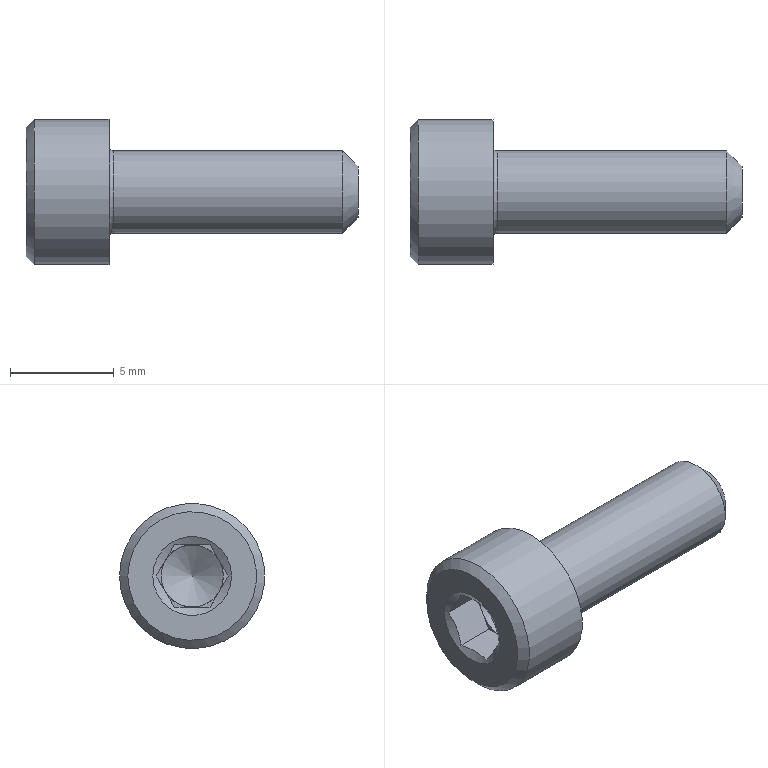Part | STEP file | Винт М4-6gx12 ГОСТ 11738-84 | 1 solid | 23 faces | box 16 x 7 x 7 mm | volume 277.854 mm3 | plane 15 | cone 4 | cylinder 3 | torus 1 | commonest cylinder face diameters 3 x1 4 x1 7 x1
STEP:
#1=CARTESIAN_POINT('',(-4.,3.1,0.));
#2=VERTEX_POINT('',#1);
#3=CARTESIAN_POINT('',(-4.,0.,0.));
#4=DIRECTION('',(1.,0.,0.));
#5=DIRECTION('',(0.,1.,0.));
#6=AXIS2_PLACEMENT_3D('',#3,#4,#5);
#7=CIRCLE('',#6,3.1);
#8=EDGE_CURVE('',#2,#2,#7,.T.);
#9=ORIENTED_EDGE('',*,*,#8,.F.);
#10=EDGE_LOOP('',(#9));
#11=FACE_BOUND('',#10,.T.);
#12=CARTESIAN_POINT('',(-4.,1.9,0.));
#13=VERTEX_POINT('',#12);
#14=CARTESIAN_POINT('',(-4.,0.,0.));
#15=DIRECTION('',(1.,0.,0.));
#16=DIRECTION('',(0.,1.,0.));
#17=AXIS2_PLACEMENT_3D('',#14,#15,#16);
#18=CIRCLE('',#17,1.9);
#19=EDGE_CURVE('',#13,#13,#18,.T.);
#20=ORIENTED_EDGE('',*,*,#19,.T.);
#21=EDGE_LOOP('',(#20));
#22=FACE_BOUND('',#21,.T.);
#23=CARTESIAN_POINT('',(-4.,0.,0.));
#24=DIRECTION('',(-1.,0.,0.));
#25=DIRECTION('',(0.,1.,0.));
#26=AXIS2_PLACEMENT_3D('',#23,#24,#25);
#27=PLANE('',#26);
#28=ADVANCED_FACE('',(#11,#22),#27,.T.);
#29=CARTESIAN_POINT('',(-3.903,0.866,-1.5));
#30=VERTEX_POINT('',#29);
#31=CARTESIAN_POINT('',(-3.903,-0.866,-1.5));
#32=VERTEX_POINT('',#31);
#33=CARTESIAN_POINT('',(-3.903,0.866,-1.5));
#34=CARTESIAN_POINT('',(-3.9,0.8561,-1.5));
#35=CARTESIAN_POINT('',(-3.89,0.8205,-1.5));
#36=CARTESIAN_POINT('',(-3.88,0.7841,-1.5));
#37=CARTESIAN_POINT('',(-3.862,0.7149,-1.5));
#38=CARTESIAN_POINT('',(-3.851,0.6675,-1.5));
#39=CARTESIAN_POINT('',(-3.83,0.5736,-1.5));
#40=CARTESIAN_POINT('',(-3.816,0.5059,-1.5));
#41=CARTESIAN_POINT('',(-3.8,0.4061,-1.5));
#42=CARTESIAN_POINT('',(-3.789,0.3305,-1.5));
#43=CARTESIAN_POINT('',(-3.781,0.2553,-1.5));
#44=CARTESIAN_POINT('',(-3.776,0.1888,-1.5));
#45=CARTESIAN_POINT('',(-3.773,0.1381,-1.5));
#46=CARTESIAN_POINT('',(-3.771,0.09396,-1.5));
#47=CARTESIAN_POINT('',(-3.77,0.0601,-1.5));
#48=CARTESIAN_POINT('',(-3.769,0.0279,-1.5));
#49=CARTESIAN_POINT('',(-3.769,-0.005342,-1.5));
#50=CARTESIAN_POINT('',(-3.769,-0.03809,-1.5));
#51=CARTESIAN_POINT('',(-3.77,-0.07339,-1.5));
#52=CARTESIAN_POINT('',(-3.771,-0.1059,-1.5));
#53=CARTESIAN_POINT('',(-3.773,-0.1382,-1.5));
#54=CARTESIAN_POINT('',(-3.775,-0.1786,-1.5));
#55=CARTESIAN_POINT('',(-3.779,-0.2268,-1.5));
#56=CARTESIAN_POINT('',(-3.783,-0.2747,-1.5));
#57=CARTESIAN_POINT('',(-3.788,-0.3143,-1.5));
#58=CARTESIAN_POINT('',(-3.792,-0.346,-1.5));
#59=CARTESIAN_POINT('',(-3.796,-0.3774,-1.5));
#60=CARTESIAN_POINT('',(-3.802,-0.4165,-1.5));
#61=CARTESIAN_POINT('',(-3.809,-0.463,-1.5));
#62=CARTESIAN_POINT('',(-3.817,-0.5065,-1.5));
#63=CARTESIAN_POINT('',(-3.823,-0.5371,-1.5));
#64=CARTESIAN_POINT('',(-3.829,-0.5675,-1.5));
#65=CARTESIAN_POINT('',(-3.836,-0.6003,-1.5));
#66=CARTESIAN_POINT('',(-3.846,-0.6453,-1.5));
#67=CARTESIAN_POINT('',(-3.856,-0.69,-1.5));
#68=CARTESIAN_POINT('',(-3.865,-0.7249,-1.5));
#69=CARTESIAN_POINT('',(-3.872,-0.7544,-1.5));
#70=CARTESIAN_POINT('',(-3.88,-0.7837,-1.5));
#71=CARTESIAN_POINT('',(-3.891,-0.8224,-1.5));
#72=CARTESIAN_POINT('',(-3.899,-0.8515,-1.5));
#73=CARTESIAN_POINT('',(-3.903,-0.866,-1.5));
#74=B_SPLINE_CURVE_WITH_KNOTS('',3,(#33,#34,#35,#36,#37,#38,#39,#40,#41,#42,#43,#44,#45,#46,#47,#48,#49,#50,#51,#52,#53,#54,#55,#56,#57,#58,#59,#60,#61,#62,#63,#64,#65,#66,#67,#68,#69,#70,#71,#72,#73),.UNSPECIFIED.,.F.,.F.,(4,1,1,1,1,1,1,1,1,1,1,1,1,1,1,1,1,1,1,1,1,1,1,1,1,1,1,1,1,1,1,1,1,1,1,1,1,1,4),(0.,0.01755,0.06316,0.06435,0.1397,0.1462,0.2284,0.2575,0.3188,0.3585,0.3865,0.4328,0.4451,0.4618,0.4905,0.5,0.5185,0.5464,0.5602,0.574,0.6016,0.6291,0.6565,0.6838,0.6972,0.7109,0.7379,0.7646,0.7912,0.8132,0.8177,0.8441,0.8703,0.8963,0.9224,0.9317,0.9483,0.9741,1.),.UNSPECIFIED.);
#75=EDGE_CURVE('',#30,#32,#74,.T.);
#76=ORIENTED_EDGE('',*,*,#75,.T.);
#77=CARTESIAN_POINT('',(-2.,-0.866,-1.5));
#78=VERTEX_POINT('',#77);
#79=CARTESIAN_POINT('',(-2.,-0.866,-1.5));
#80=DIRECTION('',(-1.,0.,0.));
#81=VECTOR('',#80,1.);
#82=LINE('',#79,#81);
#83=EDGE_CURVE('',#78,#32,#82,.T.);
#84=ORIENTED_EDGE('',*,*,#83,.F.);
#85=CARTESIAN_POINT('',(-2.,0.,-1.5));
#86=VERTEX_POINT('',#85);
#87=CARTESIAN_POINT('',(-2.,0.,-1.5));
#88=DIRECTION('',(0.,-1.,0.));
#89=VECTOR('',#88,1.);
#90=LINE('',#87,#89);
#91=EDGE_CURVE('',#86,#78,#90,.T.);
#92=ORIENTED_EDGE('',*,*,#91,.F.);
#93=CARTESIAN_POINT('',(-2.,0.866,-1.5));
#94=VERTEX_POINT('',#93);
#95=CARTESIAN_POINT('',(-2.,0.866,-1.5));
#96=DIRECTION('',(0.,-1.,0.));
#97=VECTOR('',#96,1.);
#98=LINE('',#95,#97);
#99=EDGE_CURVE('',#94,#86,#98,.T.);
#100=ORIENTED_EDGE('',*,*,#99,.F.);
#101=CARTESIAN_POINT('',(-2.,0.866,-1.5));
#102=DIRECTION('',(-1.,0.,0.));
#103=VECTOR('',#102,1.);
#104=LINE('',#101,#103);
#105=EDGE_CURVE('',#94,#30,#104,.T.);
#106=ORIENTED_EDGE('',*,*,#105,.T.);
#107=EDGE_LOOP('',(#76,#84,#92,#100,#106));
#108=FACE_BOUND('',#107,.T.);
#109=CARTESIAN_POINT('',(-2.,0.866,-1.5));
#110=DIRECTION('',(0.,0.,-1.));
#111=DIRECTION('',(0.,-1.,0.));
#112=AXIS2_PLACEMENT_3D('',#109,#110,#111);
#113=PLANE('',#112);
#114=ADVANCED_FACE('',(#108),#113,.F.);
#115=CARTESIAN_POINT('',(-3.903,-1.732,0.));
#116=VERTEX_POINT('',#115);
#117=CARTESIAN_POINT('',(-3.903,-0.866,-1.5));
#118=CARTESIAN_POINT('',(-3.893,-0.8838,-1.469));
#119=CARTESIAN_POINT('',(-3.871,-0.9233,-1.401));
#120=CARTESIAN_POINT('',(-3.839,-0.9883,-1.288));
#121=CARTESIAN_POINT('',(-3.81,-1.062,-1.161));
#122=CARTESIAN_POINT('',(-3.789,-1.133,-1.037));
#123=CARTESIAN_POINT('',(-3.777,-1.193,-0.9336));
#124=CARTESIAN_POINT('',(-3.772,-1.235,-0.8611));
#125=CARTESIAN_POINT('',(-3.77,-1.265,-0.8083));
#126=CARTESIAN_POINT('',(-3.769,-1.285,-0.7742));
#127=CARTESIAN_POINT('',(-3.769,-1.302,-0.7454));
#128=CARTESIAN_POINT('',(-3.769,-1.318,-0.717));
#129=CARTESIAN_POINT('',(-3.77,-1.34,-0.6794));
#130=CARTESIAN_POINT('',(-3.772,-1.364,-0.6373));
#131=CARTESIAN_POINT('',(-3.775,-1.388,-0.5954));
#132=CARTESIAN_POINT('',(-3.779,-1.412,-0.5536));
#133=CARTESIAN_POINT('',(-3.783,-1.436,-0.5121));
#134=CARTESIAN_POINT('',(-3.789,-1.46,-0.4709));
#135=CARTESIAN_POINT('',(-3.795,-1.484,-0.4299));
#136=CARTESIAN_POINT('',(-3.802,-1.507,-0.3893));
#137=CARTESIAN_POINT('',(-3.809,-1.531,-0.349));
#138=CARTESIAN_POINT('',(-3.817,-1.554,-0.3091));
#139=CARTESIAN_POINT('',(-3.826,-1.576,-0.2695));
#140=CARTESIAN_POINT('',(-3.836,-1.599,-0.2301));
#141=CARTESIAN_POINT('',(-3.846,-1.622,-0.1912));
#142=CARTESIAN_POINT('',(-3.856,-1.644,-0.1525));
#143=CARTESIAN_POINT('',(-3.867,-1.666,-0.114));
#144=CARTESIAN_POINT('',(-3.879,-1.688,-0.07582));
#145=CARTESIAN_POINT('',(-3.891,-1.71,-0.03781));
#146=CARTESIAN_POINT('',(-3.899,-1.725,-0.01258));
#147=CARTESIAN_POINT('',(-3.903,-1.732,0.));
#148=B_SPLINE_CURVE_WITH_KNOTS('',3,(#117,#118,#119,#120,#121,#122,#123,#124,#125,#126,#127,#128,#129,#130,#131,#132,#133,#134,#135,#136,#137,#138,#139,#140,#141,#142,#143,#144,#145,#146,#147),.UNSPECIFIED.,.F.,.F.,(4,1,1,1,1,1,1,1,1,1,1,1,1,1,1,1,1,1,1,1,1,1,1,1,1,1,1,1,4),(0.,0.06316,0.1397,0.2284,0.3188,0.3865,0.4328,0.4618,0.4905,0.5,0.5185,0.5464,0.574,0.6016,0.6291,0.6565,0.6838,0.7109,0.7379,0.7646,0.7912,0.8177,0.8441,0.8703,0.8963,0.9224,0.9483,0.9741,1.),.UNSPECIFIED.);
#149=EDGE_CURVE('',#32,#116,#148,.T.);
#150=ORIENTED_EDGE('',*,*,#149,.T.);
#151=CARTESIAN_POINT('',(-2.,-1.732,0.));
#152=VERTEX_POINT('',#151);
#153=CARTESIAN_POINT('',(-2.,-1.732,0.));
#154=DIRECTION('',(-1.,0.,0.));
#155=VECTOR('',#154,1.);
#156=LINE('',#153,#155);
#157=EDGE_CURVE('',#152,#116,#156,.T.);
#158=ORIENTED_EDGE('',*,*,#157,.F.);
#159=CARTESIAN_POINT('',(-2.,-1.299,-0.75));
#160=VERTEX_POINT('',#159);
#161=CARTESIAN_POINT('',(-2.,-1.299,-0.75));
#162=DIRECTION('',(0.,-0.5,0.866));
#163=VECTOR('',#162,1.);
#164=LINE('',#161,#163);
#165=EDGE_CURVE('',#160,#152,#164,.T.);
#166=ORIENTED_EDGE('',*,*,#165,.F.);
#167=CARTESIAN_POINT('',(-2.,-0.866,-1.5));
#168=DIRECTION('',(0.,-0.5,0.866));
#169=VECTOR('',#168,1.);
#170=LINE('',#167,#169);
#171=EDGE_CURVE('',#78,#160,#170,.T.);
#172=ORIENTED_EDGE('',*,*,#171,.F.);
#173=ORIENTED_EDGE('',*,*,#83,.T.);
#174=EDGE_LOOP('',(#150,#158,#166,#172,#173));
#175=FACE_BOUND('',#174,.T.);
#176=CARTESIAN_POINT('',(-2.,-0.866,-1.5));
#177=DIRECTION('',(0.,-0.866,-0.5));
#178=DIRECTION('',(0.,-0.5,0.866));
#179=AXIS2_PLACEMENT_3D('',#176,#177,#178);
#180=PLANE('',#179);
#181=ADVANCED_FACE('',(#175),#180,.F.);
#182=CARTESIAN_POINT('',(-3.903,-0.866,1.5));
#183=VERTEX_POINT('',#182);
#184=CARTESIAN_POINT('',(-3.903,-1.732,0.));
#185=CARTESIAN_POINT('',(-3.893,-1.714,0.0308));
#186=CARTESIAN_POINT('',(-3.871,-1.675,0.09916));
#187=CARTESIAN_POINT('',(-3.839,-1.61,0.2118));
#188=CARTESIAN_POINT('',(-3.81,-1.536,0.3391));
#189=CARTESIAN_POINT('',(-3.789,-1.465,0.4631));
#190=CARTESIAN_POINT('',(-3.777,-1.405,0.5664));
#191=CARTESIAN_POINT('',(-3.772,-1.363,0.6389));
#192=CARTESIAN_POINT('',(-3.77,-1.333,0.6917));
#193=CARTESIAN_POINT('',(-3.769,-1.313,0.7258));
#194=CARTESIAN_POINT('',(-3.769,-1.296,0.7546));
#195=CARTESIAN_POINT('',(-3.769,-1.28,0.783));
#196=CARTESIAN_POINT('',(-3.77,-1.258,0.8206));
#197=CARTESIAN_POINT('',(-3.772,-1.234,0.8627));
#198=CARTESIAN_POINT('',(-3.775,-1.21,0.9046));
#199=CARTESIAN_POINT('',(-3.779,-1.186,0.9464));
#200=CARTESIAN_POINT('',(-3.783,-1.162,0.9879));
#201=CARTESIAN_POINT('',(-3.789,-1.138,1.029));
#202=CARTESIAN_POINT('',(-3.795,-1.114,1.07));
#203=CARTESIAN_POINT('',(-3.802,-1.091,1.111));
#204=CARTESIAN_POINT('',(-3.809,-1.068,1.151));
#205=CARTESIAN_POINT('',(-3.817,-1.044,1.191));
#206=CARTESIAN_POINT('',(-3.826,-1.022,1.231));
#207=CARTESIAN_POINT('',(-3.836,-0.9989,1.27));
#208=CARTESIAN_POINT('',(-3.846,-0.9764,1.309));
#209=CARTESIAN_POINT('',(-3.856,-0.954,1.348));
#210=CARTESIAN_POINT('',(-3.867,-0.9319,1.386));
#211=CARTESIAN_POINT('',(-3.879,-0.9098,1.424));
#212=CARTESIAN_POINT('',(-3.891,-0.8879,1.462));
#213=CARTESIAN_POINT('',(-3.899,-0.8733,1.487));
#214=CARTESIAN_POINT('',(-3.903,-0.866,1.5));
#215=B_SPLINE_CURVE_WITH_KNOTS('',3,(#184,#185,#186,#187,#188,#189,#190,#191,#192,#193,#194,#195,#196,#197,#198,#199,#200,#201,#202,#203,#204,#205,#206,#207,#208,#209,#210,#211,#212,#213,#214),.UNSPECIFIED.,.F.,.F.,(4,1,1,1,1,1,1,1,1,1,1,1,1,1,1,1,1,1,1,1,1,1,1,1,1,1,1,1,4),(0.,0.06316,0.1397,0.2284,0.3188,0.3865,0.4328,0.4618,0.4905,0.5,0.5185,0.5464,0.574,0.6016,0.6291,0.6565,0.6838,0.7109,0.7379,0.7646,0.7912,0.8177,0.8441,0.8703,0.8963,0.9224,0.9483,0.9741,1.),.UNSPECIFIED.);
#216=EDGE_CURVE('',#116,#183,#215,.T.);
#217=ORIENTED_EDGE('',*,*,#216,.T.);
#218=CARTESIAN_POINT('',(-2.,-0.866,1.5));
#219=VERTEX_POINT('',#218);
#220=CARTESIAN_POINT('',(-2.,-0.866,1.5));
#221=DIRECTION('',(-1.,0.,0.));
#222=VECTOR('',#221,1.);
#223=LINE('',#220,#222);
#224=EDGE_CURVE('',#219,#183,#223,.T.);
#225=ORIENTED_EDGE('',*,*,#224,.F.);
#226=CARTESIAN_POINT('',(-2.,-1.299,0.75));
#227=VERTEX_POINT('',#226);
#228=CARTESIAN_POINT('',(-2.,-1.299,0.75));
#229=DIRECTION('',(0.,0.5,0.866));
#230=VECTOR('',#229,1.);
#231=LINE('',#228,#230);
#232=EDGE_CURVE('',#227,#219,#231,.T.);
#233=ORIENTED_EDGE('',*,*,#232,.F.);
#234=CARTESIAN_POINT('',(-2.,-1.732,0.));
#235=DIRECTION('',(0.,0.5,0.866));
#236=VECTOR('',#235,1.);
#237=LINE('',#234,#236);
#238=EDGE_CURVE('',#152,#227,#237,.T.);
#239=ORIENTED_EDGE('',*,*,#238,.F.);
#240=ORIENTED_EDGE('',*,*,#157,.T.);
#241=EDGE_LOOP('',(#217,#225,#233,#239,#240));
#242=FACE_BOUND('',#241,.T.);
#243=CARTESIAN_POINT('',(-2.,-1.732,0.));
#244=DIRECTION('',(0.,-0.866,0.5));
#245=DIRECTION('',(0.,0.5,0.866));
#246=AXIS2_PLACEMENT_3D('',#243,#244,#245);
#247=PLANE('',#246);
#248=ADVANCED_FACE('',(#242),#247,.F.);
#249=CARTESIAN_POINT('',(-3.903,0.866,1.5));
#250=VERTEX_POINT('',#249);
#251=CARTESIAN_POINT('',(-3.903,-0.866,1.5));
#252=CARTESIAN_POINT('',(-3.9,-0.8561,1.5));
#253=CARTESIAN_POINT('',(-3.89,-0.8205,1.5));
#254=CARTESIAN_POINT('',(-3.88,-0.7841,1.5));
#255=CARTESIAN_POINT('',(-3.862,-0.7149,1.5));
#256=CARTESIAN_POINT('',(-3.851,-0.6675,1.5));
#257=CARTESIAN_POINT('',(-3.83,-0.5736,1.5));
#258=CARTESIAN_POINT('',(-3.816,-0.5059,1.5));
#259=CARTESIAN_POINT('',(-3.8,-0.4061,1.5));
#260=CARTESIAN_POINT('',(-3.789,-0.3305,1.5));
#261=CARTESIAN_POINT('',(-3.781,-0.2553,1.5));
#262=CARTESIAN_POINT('',(-3.776,-0.1888,1.5));
#263=CARTESIAN_POINT('',(-3.773,-0.1381,1.5));
#264=CARTESIAN_POINT('',(-3.771,-0.09396,1.5));
#265=CARTESIAN_POINT('',(-3.77,-0.0601,1.5));
#266=CARTESIAN_POINT('',(-3.769,-0.0279,1.5));
#267=CARTESIAN_POINT('',(-3.769,0.005342,1.5));
#268=CARTESIAN_POINT('',(-3.769,0.03809,1.5));
#269=CARTESIAN_POINT('',(-3.77,0.07339,1.5));
#270=CARTESIAN_POINT('',(-3.771,0.1059,1.5));
#271=CARTESIAN_POINT('',(-3.773,0.1382,1.5));
#272=CARTESIAN_POINT('',(-3.775,0.1786,1.5));
#273=CARTESIAN_POINT('',(-3.779,0.2268,1.5));
#274=CARTESIAN_POINT('',(-3.783,0.2747,1.5));
#275=CARTESIAN_POINT('',(-3.788,0.3143,1.5));
#276=CARTESIAN_POINT('',(-3.792,0.346,1.5));
#277=CARTESIAN_POINT('',(-3.796,0.3774,1.5));
#278=CARTESIAN_POINT('',(-3.802,0.4165,1.5));
#279=CARTESIAN_POINT('',(-3.809,0.463,1.5));
#280=CARTESIAN_POINT('',(-3.817,0.5065,1.5));
#281=CARTESIAN_POINT('',(-3.823,0.5371,1.5));
#282=CARTESIAN_POINT('',(-3.829,0.5675,1.5));
#283=CARTESIAN_POINT('',(-3.836,0.6003,1.5));
#284=CARTESIAN_POINT('',(-3.846,0.6453,1.5));
#285=CARTESIAN_POINT('',(-3.856,0.69,1.5));
#286=CARTESIAN_POINT('',(-3.865,0.7249,1.5));
#287=CARTESIAN_POINT('',(-3.872,0.7544,1.5));
#288=CARTESIAN_POINT('',(-3.88,0.7837,1.5));
#289=CARTESIAN_POINT('',(-3.891,0.8224,1.5));
#290=CARTESIAN_POINT('',(-3.899,0.8515,1.5));
#291=CARTESIAN_POINT('',(-3.903,0.866,1.5));
#292=B_SPLINE_CURVE_WITH_KNOTS('',3,(#251,#252,#253,#254,#255,#256,#257,#258,#259,#260,#261,#262,#263,#264,#265,#266,#267,#268,#269,#270,#271,#272,#273,#274,#275,#276,#277,#278,#279,#280,#281,#282,#283,#284,#285,#286,#287,#288,#289,#290,#291),.UNSPECIFIED.,.F.,.F.,(4,1,1,1,1,1,1,1,1,1,1,1,1,1,1,1,1,1,1,1,1,1,1,1,1,1,1,1,1,1,1,1,1,1,1,1,1,1,4),(0.,0.01755,0.06316,0.06435,0.1397,0.1462,0.2284,0.2575,0.3188,0.3585,0.3865,0.4328,0.4451,0.4618,0.4905,0.5,0.5185,0.5464,0.5602,0.574,0.6016,0.6291,0.6565,0.6838,0.6972,0.7109,0.7379,0.7646,0.7912,0.8132,0.8177,0.8441,0.8703,0.8963,0.9224,0.9317,0.9483,0.9741,1.),.UNSPECIFIED.);
#293=EDGE_CURVE('',#183,#250,#292,.T.);
#294=ORIENTED_EDGE('',*,*,#293,.T.);
#295=CARTESIAN_POINT('',(-2.,0.866,1.5));
#296=VERTEX_POINT('',#295);
#297=CARTESIAN_POINT('',(-2.,0.866,1.5));
#298=DIRECTION('',(-1.,0.,0.));
#299=VECTOR('',#298,1.);
#300=LINE('',#297,#299);
#301=EDGE_CURVE('',#296,#250,#300,.T.);
#302=ORIENTED_EDGE('',*,*,#301,.F.);
#303=CARTESIAN_POINT('',(-2.,0.,1.5));
#304=VERTEX_POINT('',#303);
#305=CARTESIAN_POINT('',(-2.,0.,1.5));
#306=DIRECTION('',(0.,1.,0.));
#307=VECTOR('',#306,1.);
#308=LINE('',#305,#307);
#309=EDGE_CURVE('',#304,#296,#308,.T.);
#310=ORIENTED_EDGE('',*,*,#309,.F.);
#311=CARTESIAN_POINT('',(-2.,-0.866,1.5));
#312=DIRECTION('',(0.,1.,0.));
#313=VECTOR('',#312,1.);
#314=LINE('',#311,#313);
#315=EDGE_CURVE('',#219,#304,#314,.T.);
#316=ORIENTED_EDGE('',*,*,#315,.F.);
#317=ORIENTED_EDGE('',*,*,#224,.T.);
#318=EDGE_LOOP('',(#294,#302,#310,#316,#317));
#319=FACE_BOUND('',#318,.T.);
#320=CARTESIAN_POINT('',(-2.,-0.866,1.5));
#321=DIRECTION('',(0.,0.,1.));
#322=DIRECTION('',(0.,1.,0.));
#323=AXIS2_PLACEMENT_3D('',#320,#321,#322);
#324=PLANE('',#323);
#325=ADVANCED_FACE('',(#319),#324,.F.);
#326=CARTESIAN_POINT('',(-3.903,1.732,0.000000001));
#327=VERTEX_POINT('',#326);
#328=CARTESIAN_POINT('',(-3.903,1.732,0.));
#329=CARTESIAN_POINT('',(-3.893,1.714,-0.0308));
#330=CARTESIAN_POINT('',(-3.871,1.675,-0.09916));
#331=CARTESIAN_POINT('',(-3.839,1.61,-0.2118));
#332=CARTESIAN_POINT('',(-3.81,1.536,-0.3391));
#333=CARTESIAN_POINT('',(-3.789,1.465,-0.4631));
#334=CARTESIAN_POINT('',(-3.777,1.405,-0.5664));
#335=CARTESIAN_POINT('',(-3.772,1.363,-0.6389));
#336=CARTESIAN_POINT('',(-3.77,1.333,-0.6917));
#337=CARTESIAN_POINT('',(-3.769,1.313,-0.7258));
#338=CARTESIAN_POINT('',(-3.769,1.296,-0.7546));
#339=CARTESIAN_POINT('',(-3.769,1.28,-0.783));
#340=CARTESIAN_POINT('',(-3.77,1.258,-0.8206));
#341=CARTESIAN_POINT('',(-3.772,1.234,-0.8627));
#342=CARTESIAN_POINT('',(-3.775,1.21,-0.9046));
#343=CARTESIAN_POINT('',(-3.779,1.186,-0.9464));
#344=CARTESIAN_POINT('',(-3.783,1.162,-0.9879));
#345=CARTESIAN_POINT('',(-3.789,1.138,-1.029));
#346=CARTESIAN_POINT('',(-3.795,1.114,-1.07));
#347=CARTESIAN_POINT('',(-3.802,1.091,-1.111));
#348=CARTESIAN_POINT('',(-3.809,1.068,-1.151));
#349=CARTESIAN_POINT('',(-3.817,1.044,-1.191));
#350=CARTESIAN_POINT('',(-3.826,1.022,-1.231));
#351=CARTESIAN_POINT('',(-3.836,0.9989,-1.27));
#352=CARTESIAN_POINT('',(-3.846,0.9764,-1.309));
#353=CARTESIAN_POINT('',(-3.856,0.954,-1.348));
#354=CARTESIAN_POINT('',(-3.867,0.9319,-1.386));
#355=CARTESIAN_POINT('',(-3.879,0.9098,-1.424));
#356=CARTESIAN_POINT('',(-3.891,0.8879,-1.462));
#357=CARTESIAN_POINT('',(-3.899,0.8733,-1.487));
#358=CARTESIAN_POINT('',(-3.903,0.866,-1.5));
#359=B_SPLINE_CURVE_WITH_KNOTS('',3,(#328,#329,#330,#331,#332,#333,#334,#335,#336,#337,#338,#339,#340,#341,#342,#343,#344,#345,#346,#347,#348,#349,#350,#351,#352,#353,#354,#355,#356,#357,#358),.UNSPECIFIED.,.F.,.F.,(4,1,1,1,1,1,1,1,1,1,1,1,1,1,1,1,1,1,1,1,1,1,1,1,1,1,1,1,4),(0.,0.06315,0.1397,0.2284,0.3188,0.3865,0.4327,0.4618,0.4905,0.5,0.5185,0.5464,0.574,0.6016,0.6291,0.6565,0.6838,0.7109,0.7379,0.7646,0.7912,0.8177,0.8441,0.8703,0.8963,0.9224,0.9483,0.9741,1.),.UNSPECIFIED.);
#360=EDGE_CURVE('',#327,#30,#359,.T.);
#361=ORIENTED_EDGE('',*,*,#360,.T.);
#362=ORIENTED_EDGE('',*,*,#105,.F.);
#363=CARTESIAN_POINT('',(-2.,1.299,-0.75));
#364=VERTEX_POINT('',#363);
#365=CARTESIAN_POINT('',(-2.,1.299,-0.75));
#366=DIRECTION('',(0.,-0.5,-0.866));
#367=VECTOR('',#366,1.);
#368=LINE('',#365,#367);
#369=EDGE_CURVE('',#364,#94,#368,.T.);
#370=ORIENTED_EDGE('',*,*,#369,.F.);
#371=CARTESIAN_POINT('',(-2.,1.732,0.));
#372=VERTEX_POINT('',#371);
#373=CARTESIAN_POINT('',(-2.,1.732,0.));
#374=DIRECTION('',(0.,-0.5,-0.866));
#375=VECTOR('',#374,1.);
#376=LINE('',#373,#375);
#377=EDGE_CURVE('',#372,#364,#376,.T.);
#378=ORIENTED_EDGE('',*,*,#377,.F.);
#379=CARTESIAN_POINT('',(-2.,1.732,0.));
#380=DIRECTION('',(-1.,0.,0.));
#381=VECTOR('',#380,1.);
#382=LINE('',#379,#381);
#383=EDGE_CURVE('',#372,#327,#382,.T.);
#384=ORIENTED_EDGE('',*,*,#383,.T.);
#385=EDGE_LOOP('',(#361,#362,#370,#378,#384));
#386=FACE_BOUND('',#385,.T.);
#387=CARTESIAN_POINT('',(-2.,1.732,0.));
#388=DIRECTION('',(0.,0.866,-0.5));
#389=DIRECTION('',(0.,-0.5,-0.866));
#390=AXIS2_PLACEMENT_3D('',#387,#388,#389);
#391=PLANE('',#390);
#392=ADVANCED_FACE('',(#386),#391,.F.);
#393=CARTESIAN_POINT('',(-3.903,0.866,1.5));
#394=CARTESIAN_POINT('',(-3.893,0.8838,1.469));
#395=CARTESIAN_POINT('',(-3.871,0.9233,1.401));
#396=CARTESIAN_POINT('',(-3.839,0.9883,1.288));
#397=CARTESIAN_POINT('',(-3.81,1.062,1.161));
#398=CARTESIAN_POINT('',(-3.789,1.133,1.037));
#399=CARTESIAN_POINT('',(-3.777,1.193,0.9336));
#400=CARTESIAN_POINT('',(-3.772,1.235,0.8611));
#401=CARTESIAN_POINT('',(-3.77,1.265,0.8083));
#402=CARTESIAN_POINT('',(-3.769,1.285,0.7742));
#403=CARTESIAN_POINT('',(-3.769,1.302,0.7454));
#404=CARTESIAN_POINT('',(-3.769,1.318,0.717));
#405=CARTESIAN_POINT('',(-3.77,1.34,0.6794));
#406=CARTESIAN_POINT('',(-3.772,1.364,0.6373));
#407=CARTESIAN_POINT('',(-3.775,1.388,0.5954));
#408=CARTESIAN_POINT('',(-3.779,1.412,0.5536));
#409=CARTESIAN_POINT('',(-3.783,1.436,0.5121));
#410=CARTESIAN_POINT('',(-3.789,1.46,0.4709));
#411=CARTESIAN_POINT('',(-3.795,1.484,0.4299));
#412=CARTESIAN_POINT('',(-3.802,1.507,0.3893));
#413=CARTESIAN_POINT('',(-3.809,1.531,0.349));
#414=CARTESIAN_POINT('',(-3.817,1.554,0.3091));
#415=CARTESIAN_POINT('',(-3.826,1.576,0.2695));
#416=CARTESIAN_POINT('',(-3.836,1.599,0.2301));
#417=CARTESIAN_POINT('',(-3.846,1.622,0.1912));
#418=CARTESIAN_POINT('',(-3.856,1.644,0.1525));
#419=CARTESIAN_POINT('',(-3.867,1.666,0.114));
#420=CARTESIAN_POINT('',(-3.879,1.688,0.07582));
#421=CARTESIAN_POINT('',(-3.891,1.71,0.03781));
#422=CARTESIAN_POINT('',(-3.899,1.725,0.01258));
#423=CARTESIAN_POINT('',(-3.903,1.732,0.000000005));
#424=B_SPLINE_CURVE_WITH_KNOTS('',3,(#393,#394,#395,#396,#397,#398,#399,#400,#401,#402,#403,#404,#405,#406,#407,#408,#409,#410,#411,#412,#413,#414,#415,#416,#417,#418,#419,#420,#421,#422,#423),.UNSPECIFIED.,.F.,.F.,(4,1,1,1,1,1,1,1,1,1,1,1,1,1,1,1,1,1,1,1,1,1,1,1,1,1,1,1,4),(0.,0.06315,0.1397,0.2284,0.3188,0.3865,0.4327,0.4618,0.4905,0.5,0.5185,0.5464,0.574,0.6016,0.6291,0.6565,0.6838,0.7109,0.7379,0.7646,0.7912,0.8177,0.8441,0.8703,0.8963,0.9224,0.9483,0.9741,1.),.UNSPECIFIED.);
#425=EDGE_CURVE('',#250,#327,#424,.T.);
#426=ORIENTED_EDGE('',*,*,#425,.T.);
#427=ORIENTED_EDGE('',*,*,#383,.F.);
#428=CARTESIAN_POINT('',(-2.,1.299,0.75));
#429=VERTEX_POINT('',#428);
#430=CARTESIAN_POINT('',(-2.,1.299,0.75));
#431=DIRECTION('',(0.,0.5,-0.866));
#432=VECTOR('',#431,1.);
#433=LINE('',#430,#432);
#434=EDGE_CURVE('',#429,#372,#433,.T.);
#435=ORIENTED_EDGE('',*,*,#434,.F.);
#436=CARTESIAN_POINT('',(-2.,0.866,1.5));
#437=DIRECTION('',(0.,0.5,-0.866));
#438=VECTOR('',#437,1.);
#439=LINE('',#436,#438);
#440=EDGE_CURVE('',#296,#429,#439,.T.);
#441=ORIENTED_EDGE('',*,*,#440,.F.);
#442=ORIENTED_EDGE('',*,*,#301,.T.);
#443=EDGE_LOOP('',(#426,#427,#435,#441,#442));
#444=FACE_BOUND('',#443,.T.);
#445=CARTESIAN_POINT('',(-2.,0.866,1.5));
#446=DIRECTION('',(0.,0.866,0.5));
#447=DIRECTION('',(0.,0.5,-0.866));
#448=AXIS2_PLACEMENT_3D('',#445,#446,#447);
#449=PLANE('',#448);
#450=ADVANCED_FACE('',(#444),#449,.F.);
#451=ORIENTED_EDGE('',*,*,#425,.F.);
#452=ORIENTED_EDGE('',*,*,#293,.F.);
#453=ORIENTED_EDGE('',*,*,#216,.F.);
#454=ORIENTED_EDGE('',*,*,#149,.F.);
#455=ORIENTED_EDGE('',*,*,#75,.F.);
#456=ORIENTED_EDGE('',*,*,#360,.F.);
#457=EDGE_LOOP('',(#451,#452,#453,#454,#455,#456));
#458=FACE_BOUND('',#457,.T.);
#459=ORIENTED_EDGE('',*,*,#19,.F.);
#460=EDGE_LOOP('',(#459));
#461=FACE_OUTER_BOUND('',#460,.T.);
#462=CARTESIAN_POINT('',(-3.885,0.,0.));
#463=DIRECTION('',(-1.,0.,0.));
#464=DIRECTION('',(0.,-1.,0.));
#465=AXIS2_PLACEMENT_3D('',#462,#463,#464);
#466=CONICAL_SURFACE('',#465,1.7,1.047);
#467=ADVANCED_FACE('',(#458,#461),#466,.F.);
#468=CARTESIAN_POINT('',(-3.6,3.5,0.));
#469=VERTEX_POINT('',#468);
#470=CARTESIAN_POINT('',(-3.6,0.,0.));
#471=DIRECTION('',(1.,0.,0.));
#472=DIRECTION('',(0.,1.,0.));
#473=AXIS2_PLACEMENT_3D('',#470,#471,#472);
#474=CIRCLE('',#473,3.5);
#475=EDGE_CURVE('',#469,#469,#474,.T.);
#476=ORIENTED_EDGE('',*,*,#475,.F.);
#477=EDGE_LOOP('',(#476));
#478=FACE_OUTER_BOUND('',#477,.T.);
#479=ORIENTED_EDGE('',*,*,#8,.T.);
#480=EDGE_LOOP('',(#479));
#481=FACE_OUTER_BOUND('',#480,.T.);
#482=CARTESIAN_POINT('',(-3.8,0.,0.));
#483=DIRECTION('',(1.,0.,0.));
#484=DIRECTION('',(0.,1.,0.));
#485=AXIS2_PLACEMENT_3D('',#482,#483,#484);
#486=CONICAL_SURFACE('',#485,3.3,0.7854);
#487=ADVANCED_FACE('',(#478,#481),#486,.T.);
#488=CARTESIAN_POINT('',(-2.,0.,0.));
#489=DIRECTION('',(1.,0.,0.));
#490=DIRECTION('',(0.,-0.866,-0.5));
#491=AXIS2_PLACEMENT_3D('',#488,#489,#490);
#492=CIRCLE('',#491,1.5);
#493=EDGE_CURVE('',#160,#86,#492,.T.);
#494=ORIENTED_EDGE('',*,*,#493,.T.);
#495=ORIENTED_EDGE('',*,*,#91,.T.);
#496=ORIENTED_EDGE('',*,*,#171,.T.);
#497=EDGE_LOOP('',(#494,#495,#496));
#498=FACE_BOUND('',#497,.T.);
#499=CARTESIAN_POINT('',(-2.,0.,0.));
#500=DIRECTION('',(-1.,0.,0.));
#501=DIRECTION('',(0.,0.,-1.));
#502=AXIS2_PLACEMENT_3D('',#499,#500,#501);
#503=PLANE('',#502);
#504=ADVANCED_FACE('',(#498),#503,.T.);
#505=CARTESIAN_POINT('',(-2.,0.,0.));
#506=DIRECTION('',(1.,0.,0.));
#507=DIRECTION('',(0.,0.,-1.));
#508=AXIS2_PLACEMENT_3D('',#505,#506,#507);
#509=CIRCLE('',#508,1.5);
#510=EDGE_CURVE('',#86,#364,#509,.T.);
#511=ORIENTED_EDGE('',*,*,#510,.T.);
#512=ORIENTED_EDGE('',*,*,#369,.T.);
#513=ORIENTED_EDGE('',*,*,#99,.T.);
#514=EDGE_LOOP('',(#511,#512,#513));
#515=FACE_BOUND('',#514,.T.);
#516=CARTESIAN_POINT('',(-2.,0.,0.));
#517=DIRECTION('',(-1.,0.,0.));
#518=DIRECTION('',(0.,0.,-1.));
#519=AXIS2_PLACEMENT_3D('',#516,#517,#518);
#520=PLANE('',#519);
#521=ADVANCED_FACE('',(#515),#520,.T.);
#522=CARTESIAN_POINT('',(-2.,0.,0.));
#523=DIRECTION('',(1.,0.,0.));
#524=DIRECTION('',(0.,-0.866,0.5));
#525=AXIS2_PLACEMENT_3D('',#522,#523,#524);
#526=CIRCLE('',#525,1.5);
#527=EDGE_CURVE('',#227,#160,#526,.T.);
#528=ORIENTED_EDGE('',*,*,#527,.T.);
#529=ORIENTED_EDGE('',*,*,#165,.T.);
#530=ORIENTED_EDGE('',*,*,#238,.T.);
#531=EDGE_LOOP('',(#528,#529,#530));
#532=FACE_BOUND('',#531,.T.);
#533=CARTESIAN_POINT('',(-2.,0.,0.));
#534=DIRECTION('',(-1.,0.,0.));
#535=DIRECTION('',(0.,0.,-1.));
#536=AXIS2_PLACEMENT_3D('',#533,#534,#535);
#537=PLANE('',#536);
#538=ADVANCED_FACE('',(#532),#537,.T.);
#539=CARTESIAN_POINT('',(-2.,0.,0.));
#540=DIRECTION('',(1.,0.,0.));
#541=DIRECTION('',(0.,0.,1.));
#542=AXIS2_PLACEMENT_3D('',#539,#540,#541);
#543=CIRCLE('',#542,1.5);
#544=EDGE_CURVE('',#304,#227,#543,.T.);
#545=ORIENTED_EDGE('',*,*,#544,.T.);
#546=ORIENTED_EDGE('',*,*,#232,.T.);
#547=ORIENTED_EDGE('',*,*,#315,.T.);
#548=EDGE_LOOP('',(#545,#546,#547));
#549=FACE_BOUND('',#548,.T.);
#550=CARTESIAN_POINT('',(-2.,0.,0.));
#551=DIRECTION('',(-1.,0.,0.));
#552=DIRECTION('',(0.,0.,-1.));
#553=AXIS2_PLACEMENT_3D('',#550,#551,#552);
#554=PLANE('',#553);
#555=ADVANCED_FACE('',(#549),#554,.T.);
#556=CARTESIAN_POINT('',(-2.,0.,0.));
#557=DIRECTION('',(1.,0.,0.));
#558=DIRECTION('',(0.,0.866,0.5));
#559=AXIS2_PLACEMENT_3D('',#556,#557,#558);
#560=CIRCLE('',#559,1.5);
#561=EDGE_CURVE('',#429,#304,#560,.T.);
#562=ORIENTED_EDGE('',*,*,#561,.T.);
#563=ORIENTED_EDGE('',*,*,#309,.T.);
#564=ORIENTED_EDGE('',*,*,#440,.T.);
#565=EDGE_LOOP('',(#562,#563,#564));
#566=FACE_BOUND('',#565,.T.);
#567=CARTESIAN_POINT('',(-2.,0.,0.));
#568=DIRECTION('',(-1.,0.,0.));
#569=DIRECTION('',(0.,0.,-1.));
#570=AXIS2_PLACEMENT_3D('',#567,#568,#569);
#571=PLANE('',#570);
#572=ADVANCED_FACE('',(#566),#571,.T.);
#573=CARTESIAN_POINT('',(-2.,1.5,0.));
#574=VERTEX_POINT('',#573);
#575=CARTESIAN_POINT('',(-2.,0.,0.));
#576=DIRECTION('',(1.,0.,0.));
#577=DIRECTION('',(0.,1.,0.));
#578=AXIS2_PLACEMENT_3D('',#575,#576,#577);
#579=CIRCLE('',#578,1.5);
#580=EDGE_CURVE('',#574,#429,#579,.T.);
#581=ORIENTED_EDGE('',*,*,#580,.T.);
#582=ORIENTED_EDGE('',*,*,#434,.T.);
#583=ORIENTED_EDGE('',*,*,#377,.T.);
#584=CARTESIAN_POINT('',(-2.,0.,0.));
#585=DIRECTION('',(1.,0.,0.));
#586=DIRECTION('',(0.,0.866,-0.5));
#587=AXIS2_PLACEMENT_3D('',#584,#585,#586);
#588=CIRCLE('',#587,1.5);
#589=EDGE_CURVE('',#364,#574,#588,.T.);
#590=ORIENTED_EDGE('',*,*,#589,.T.);
#591=EDGE_LOOP('',(#581,#582,#583,#590));
#592=FACE_BOUND('',#591,.T.);
#593=CARTESIAN_POINT('',(-2.,0.,0.));
#594=DIRECTION('',(-1.,0.,0.));
#595=DIRECTION('',(0.,0.,-1.));
#596=AXIS2_PLACEMENT_3D('',#593,#594,#595);
#597=PLANE('',#596);
#598=ADVANCED_FACE('',(#592),#597,.T.);
#599=CARTESIAN_POINT('',(0.,3.5,0.));
#600=VERTEX_POINT('',#599);
#601=CARTESIAN_POINT('',(0.,0.,0.));
#602=DIRECTION('',(1.,0.,0.));
#603=DIRECTION('',(0.,1.,0.));
#604=AXIS2_PLACEMENT_3D('',#601,#602,#603);
#605=CIRCLE('',#604,3.5);
#606=EDGE_CURVE('',#600,#600,#605,.T.);
#607=ORIENTED_EDGE('',*,*,#606,.F.);
#608=EDGE_LOOP('',(#607));
#609=FACE_OUTER_BOUND('',#608,.T.);
#610=ORIENTED_EDGE('',*,*,#475,.T.);
#611=EDGE_LOOP('',(#610));
#612=FACE_OUTER_BOUND('',#611,.T.);
#613=CARTESIAN_POINT('',(-4.,0.,0.));
#614=DIRECTION('',(1.,0.,0.));
#615=DIRECTION('',(0.,1.,0.));
#616=AXIS2_PLACEMENT_3D('',#613,#614,#615);
#617=CYLINDRICAL_SURFACE('',#616,3.5);
#618=ADVANCED_FACE('',(#609,#612),#617,.T.);
#619=CARTESIAN_POINT('',(-1.4,1.5,0.));
#620=VERTEX_POINT('',#619);
#621=CARTESIAN_POINT('',(-1.4,0.,0.));
#622=DIRECTION('',(1.,0.,0.));
#623=DIRECTION('',(0.,1.,0.));
#624=AXIS2_PLACEMENT_3D('',#621,#622,#623);
#625=CIRCLE('',#624,1.5);
#626=EDGE_CURVE('',#620,#620,#625,.T.);
#627=ORIENTED_EDGE('',*,*,#626,.T.);
#628=EDGE_LOOP('',(#627));
#629=FACE_OUTER_BOUND('',#628,.T.);
#630=ORIENTED_EDGE('',*,*,#589,.F.);
#631=ORIENTED_EDGE('',*,*,#510,.F.);
#632=ORIENTED_EDGE('',*,*,#493,.F.);
#633=ORIENTED_EDGE('',*,*,#527,.F.);
#634=ORIENTED_EDGE('',*,*,#544,.F.);
#635=ORIENTED_EDGE('',*,*,#561,.F.);
#636=ORIENTED_EDGE('',*,*,#580,.F.);
#637=EDGE_LOOP('',(#630,#631,#632,#633,#634,#635,#636));
#638=FACE_BOUND('',#637,.T.);
#639=CARTESIAN_POINT('',(-4.,0.,0.));
#640=DIRECTION('',(1.,0.,0.));
#641=DIRECTION('',(0.,1.,0.));
#642=AXIS2_PLACEMENT_3D('',#639,#640,#641);
#643=CYLINDRICAL_SURFACE('',#642,1.5);
#644=ADVANCED_FACE('',(#629,#638),#643,.F.);
#645=ORIENTED_EDGE('',*,*,#606,.T.);
#646=EDGE_LOOP('',(#645));
#647=FACE_BOUND('',#646,.T.);
#648=CARTESIAN_POINT('',(0.,0.,-2.2));
#649=VERTEX_POINT('',#648);
#650=CARTESIAN_POINT('',(0.,0.,0.));
#651=DIRECTION('',(-1.,0.,0.));
#652=DIRECTION('',(0.,0.,-1.));
#653=AXIS2_PLACEMENT_3D('',#650,#651,#652);
#654=CIRCLE('',#653,2.2);
#655=EDGE_CURVE('',#649,#649,#654,.T.);
#656=ORIENTED_EDGE('',*,*,#655,.T.);
#657=EDGE_LOOP('',(#656));
#658=FACE_BOUND('',#657,.T.);
#659=CARTESIAN_POINT('',(0.,0.,0.));
#660=DIRECTION('',(1.,0.,0.));
#661=DIRECTION('',(0.,1.,0.));
#662=AXIS2_PLACEMENT_3D('',#659,#660,#661);
#663=PLANE('',#662);
#664=ADVANCED_FACE('',(#647,#658),#663,.T.);
#665=ORIENTED_EDGE('',*,*,#626,.F.);
#666=EDGE_LOOP('',(#665));
#667=FACE_OUTER_BOUND('',#666,.T.);
#668=CARTESIAN_POINT('',(-0.967,0.,0.));
#669=DIRECTION('',(-1.,0.,0.));
#670=DIRECTION('',(0.,-1.,0.));
#671=AXIS2_PLACEMENT_3D('',#668,#669,#670);
#672=CONICAL_SURFACE('',#671,0.75,1.047);
#673=ADVANCED_FACE('',(#667),#672,.F.);
#674=CARTESIAN_POINT('',(0.2,0.,-2.));
#675=VERTEX_POINT('',#674);
#676=CARTESIAN_POINT('',(0.2,0.,0.));
#677=DIRECTION('',(-1.,0.,0.));
#678=DIRECTION('',(0.,0.,-1.));
#679=AXIS2_PLACEMENT_3D('',#676,#677,#678);
#680=CIRCLE('',#679,2.);
#681=EDGE_CURVE('',#675,#675,#680,.T.);
#682=ORIENTED_EDGE('',*,*,#681,.T.);
#683=EDGE_LOOP('',(#682));
#684=FACE_OUTER_BOUND('',#683,.T.);
#685=ORIENTED_EDGE('',*,*,#655,.F.);
#686=EDGE_LOOP('',(#685));
#687=FACE_OUTER_BOUND('',#686,.T.);
#688=CARTESIAN_POINT('',(0.2,0.,0.));
#689=DIRECTION('',(-1.,0.,0.));
#690=DIRECTION('',(0.,0.,-1.));
#691=AXIS2_PLACEMENT_3D('',#688,#689,#690);
#692=TOROIDAL_SURFACE('',#691,2.2,0.2);
#693=ADVANCED_FACE('',(#684,#687),#692,.F.);
#694=CARTESIAN_POINT('',(11.25,0.,-2.));
#695=VERTEX_POINT('',#694);
#696=CARTESIAN_POINT('',(11.25,0.,0.));
#697=DIRECTION('',(-1.,0.,0.));
#698=DIRECTION('',(0.,0.,-1.));
#699=AXIS2_PLACEMENT_3D('',#696,#697,#698);
#700=CIRCLE('',#699,2.);
#701=EDGE_CURVE('',#695,#695,#700,.T.);
#702=ORIENTED_EDGE('',*,*,#701,.T.);
#703=EDGE_LOOP('',(#702));
#704=FACE_OUTER_BOUND('',#703,.T.);
#705=ORIENTED_EDGE('',*,*,#681,.F.);
#706=EDGE_LOOP('',(#705));
#707=FACE_OUTER_BOUND('',#706,.T.);
#708=CARTESIAN_POINT('',(12.,0.,0.));
#709=DIRECTION('',(-1.,0.,0.));
#710=DIRECTION('',(0.,0.,-1.));
#711=AXIS2_PLACEMENT_3D('',#708,#709,#710);
#712=CYLINDRICAL_SURFACE('',#711,2.);
#713=ADVANCED_FACE('',(#704,#707),#712,.T.);
#714=CARTESIAN_POINT('',(12.,0.,-1.25));
#715=VERTEX_POINT('',#714);
#716=CARTESIAN_POINT('',(12.,0.,0.));
#717=DIRECTION('',(-1.,0.,0.));
#718=DIRECTION('',(0.,0.,-1.));
#719=AXIS2_PLACEMENT_3D('',#716,#717,#718);
#720=CIRCLE('',#719,1.25);
#721=EDGE_CURVE('',#715,#715,#720,.T.);
#722=ORIENTED_EDGE('',*,*,#721,.F.);
#723=EDGE_LOOP('',(#722));
#724=FACE_BOUND('',#723,.T.);
#725=CARTESIAN_POINT('',(12.,0.,0.));
#726=DIRECTION('',(-1.,0.,0.));
#727=DIRECTION('',(0.,0.,-1.));
#728=AXIS2_PLACEMENT_3D('',#725,#726,#727);
#729=PLANE('',#728);
#730=ADVANCED_FACE('',(#724),#729,.F.);
#731=ORIENTED_EDGE('',*,*,#721,.T.);
#732=EDGE_LOOP('',(#731));
#733=FACE_OUTER_BOUND('',#732,.T.);
#734=ORIENTED_EDGE('',*,*,#701,.F.);
#735=EDGE_LOOP('',(#734));
#736=FACE_OUTER_BOUND('',#735,.T.);
#737=CARTESIAN_POINT('',(11.625,0.,0.));
#738=DIRECTION('',(-1.,0.,0.));
#739=DIRECTION('',(0.,0.,-1.));
#740=AXIS2_PLACEMENT_3D('',#737,#738,#739);
#741=CONICAL_SURFACE('',#740,1.625,0.7854);
#742=ADVANCED_FACE('',(#733,#736),#741,.T.);
#743=CLOSED_SHELL('',(#28,#114,#181,#248,#325,#392,#450,#467,#487,#504,#521,#538,#555,#572,#598,#618,#644,#664,#673,#693,#713,#730,#742));
#744=MANIFOLD_SOLID_BREP('',#743);
#745=(LENGTH_UNIT()NAMED_UNIT(*)SI_UNIT(.MILLI.,.METRE.));
#746=UNCERTAINTY_MEASURE_WITH_UNIT(LENGTH_MEASURE(0.00001),#745,'','');
#747=(NAMED_UNIT(*)PLANE_ANGLE_UNIT()SI_UNIT($,.RADIAN.));
#748=(NAMED_UNIT(*)SI_UNIT($,.STERADIAN.)SOLID_ANGLE_UNIT());
#749=(GEOMETRIC_REPRESENTATION_CONTEXT(3)GLOBAL_UNCERTAINTY_ASSIGNED_CONTEXT((#746))GLOBAL_UNIT_ASSIGNED_CONTEXT((#745,#747,#748))REPRESENTATION_CONTEXT('',''));
#750=ADVANCED_BREP_SHAPE_REPRESENTATION('',(#744),#749);